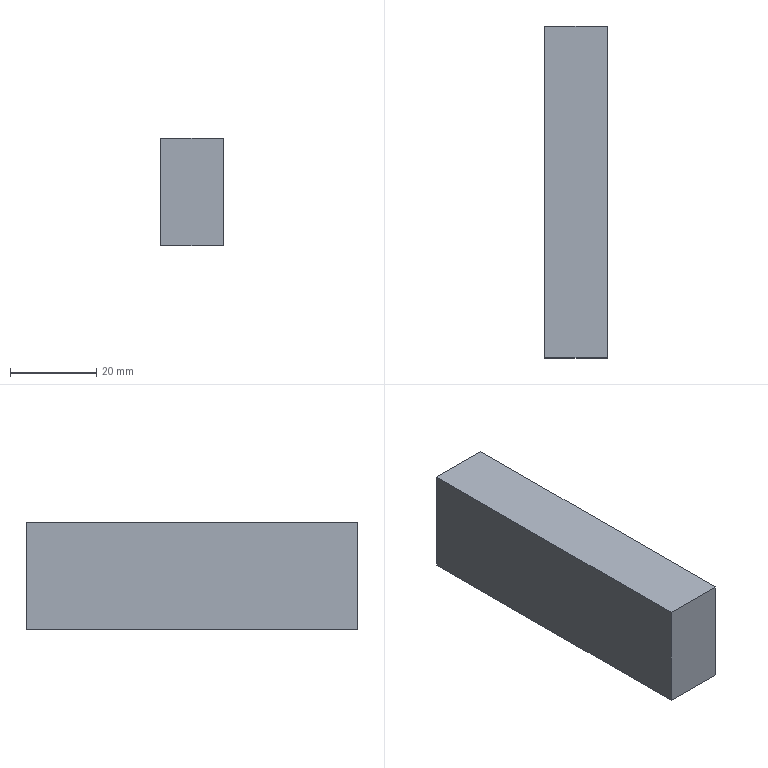Part | SolidWorks | features Extrusion 1 | 1 solid | 6 faces | box 14.5 x 77 x 25 mm | volume 27913 mm3 | plane 6
STEP:
#1=CARTESIAN_POINT('',(-7.25,38.5,0.));
#2=VERTEX_POINT('',#1);
#3=CARTESIAN_POINT('',(-7.25,-38.5,0.));
#4=VERTEX_POINT('',#3);
#5=CARTESIAN_POINT('',(-7.25,-38.5,0.));
#6=DIRECTION('',(0.,-1.,0.));
#7=VECTOR('',#6,1000.);
#8=LINE('',#5,#7);
#9=EDGE_CURVE('',#2,#4,#8,.T.);
#10=ORIENTED_EDGE('',*,*,#9,.T.);
#11=CARTESIAN_POINT('',(-7.25,-38.5,25.));
#12=VERTEX_POINT('',#11);
#13=CARTESIAN_POINT('',(-7.25,-38.5,25.));
#14=DIRECTION('',(0.,0.,-1.));
#15=VECTOR('',#14,1000.);
#16=LINE('',#13,#15);
#17=EDGE_CURVE('',#12,#4,#16,.T.);
#18=ORIENTED_EDGE('',*,*,#17,.F.);
#19=CARTESIAN_POINT('',(-7.25,38.5,25.));
#20=VERTEX_POINT('',#19);
#21=CARTESIAN_POINT('',(-7.25,-38.5,25.));
#22=DIRECTION('',(0.,-1.,0.));
#23=VECTOR('',#22,1000.);
#24=LINE('',#21,#23);
#25=EDGE_CURVE('',#20,#12,#24,.T.);
#26=ORIENTED_EDGE('',*,*,#25,.F.);
#27=CARTESIAN_POINT('',(-7.25,38.5,25.));
#28=DIRECTION('',(0.,0.,-1.));
#29=VECTOR('',#28,1000.);
#30=LINE('',#27,#29);
#31=EDGE_CURVE('',#20,#2,#30,.T.);
#32=ORIENTED_EDGE('',*,*,#31,.T.);
#33=EDGE_LOOP('',(#10,#18,#26,#32));
#34=FACE_OUTER_BOUND('',#33,.T.);
#35=CARTESIAN_POINT('',(-7.25,-38.5,25.));
#36=DIRECTION('',(1.,0.,0.));
#37=DIRECTION('',(0.,1.,0.));
#38=AXIS2_PLACEMENT_3D('',#35,#36,#37);
#39=PLANE('',#38);
#40=ADVANCED_FACE('',(#34),#39,.F.);
#41=CARTESIAN_POINT('',(7.25,-38.5,0.));
#42=VERTEX_POINT('',#41);
#43=CARTESIAN_POINT('',(7.25,-38.5,0.));
#44=DIRECTION('',(1.,0.,0.));
#45=VECTOR('',#44,1000.);
#46=LINE('',#43,#45);
#47=EDGE_CURVE('',#4,#42,#46,.T.);
#48=ORIENTED_EDGE('',*,*,#47,.T.);
#49=CARTESIAN_POINT('',(7.25,-38.5,25.));
#50=VERTEX_POINT('',#49);
#51=CARTESIAN_POINT('',(7.25,-38.5,25.));
#52=DIRECTION('',(0.,0.,-1.));
#53=VECTOR('',#52,1000.);
#54=LINE('',#51,#53);
#55=EDGE_CURVE('',#50,#42,#54,.T.);
#56=ORIENTED_EDGE('',*,*,#55,.F.);
#57=CARTESIAN_POINT('',(7.25,-38.5,25.));
#58=DIRECTION('',(1.,0.,0.));
#59=VECTOR('',#58,1000.);
#60=LINE('',#57,#59);
#61=EDGE_CURVE('',#12,#50,#60,.T.);
#62=ORIENTED_EDGE('',*,*,#61,.F.);
#63=ORIENTED_EDGE('',*,*,#17,.T.);
#64=EDGE_LOOP('',(#48,#56,#62,#63));
#65=FACE_OUTER_BOUND('',#64,.T.);
#66=CARTESIAN_POINT('',(7.25,-38.5,25.));
#67=DIRECTION('',(0.,1.,0.));
#68=DIRECTION('',(0.,0.,1.));
#69=AXIS2_PLACEMENT_3D('',#66,#67,#68);
#70=PLANE('',#69);
#71=ADVANCED_FACE('',(#65),#70,.F.);
#72=CARTESIAN_POINT('',(7.25,38.5,0.));
#73=VERTEX_POINT('',#72);
#74=CARTESIAN_POINT('',(7.25,-38.5,0.));
#75=DIRECTION('',(0.,1.,0.));
#76=VECTOR('',#75,1000.);
#77=LINE('',#74,#76);
#78=EDGE_CURVE('',#42,#73,#77,.T.);
#79=ORIENTED_EDGE('',*,*,#78,.T.);
#80=CARTESIAN_POINT('',(7.25,38.5,25.));
#81=VERTEX_POINT('',#80);
#82=CARTESIAN_POINT('',(7.25,38.5,25.));
#83=DIRECTION('',(0.,0.,-1.));
#84=VECTOR('',#83,1000.);
#85=LINE('',#82,#84);
#86=EDGE_CURVE('',#81,#73,#85,.T.);
#87=ORIENTED_EDGE('',*,*,#86,.F.);
#88=CARTESIAN_POINT('',(7.25,-38.5,25.));
#89=DIRECTION('',(0.,1.,0.));
#90=VECTOR('',#89,1000.);
#91=LINE('',#88,#90);
#92=EDGE_CURVE('',#50,#81,#91,.T.);
#93=ORIENTED_EDGE('',*,*,#92,.F.);
#94=ORIENTED_EDGE('',*,*,#55,.T.);
#95=EDGE_LOOP('',(#79,#87,#93,#94));
#96=FACE_OUTER_BOUND('',#95,.T.);
#97=CARTESIAN_POINT('',(7.25,-38.5,25.));
#98=DIRECTION('',(-1.,0.,0.));
#99=DIRECTION('',(0.,0.,1.));
#100=AXIS2_PLACEMENT_3D('',#97,#98,#99);
#101=PLANE('',#100);
#102=ADVANCED_FACE('',(#96),#101,.F.);
#103=CARTESIAN_POINT('',(7.25,38.5,0.));
#104=DIRECTION('',(-1.,0.,0.));
#105=VECTOR('',#104,1000.);
#106=LINE('',#103,#105);
#107=EDGE_CURVE('',#73,#2,#106,.T.);
#108=ORIENTED_EDGE('',*,*,#107,.T.);
#109=ORIENTED_EDGE('',*,*,#31,.F.);
#110=CARTESIAN_POINT('',(7.25,38.5,25.));
#111=DIRECTION('',(-1.,0.,0.));
#112=VECTOR('',#111,1000.);
#113=LINE('',#110,#112);
#114=EDGE_CURVE('',#81,#20,#113,.T.);
#115=ORIENTED_EDGE('',*,*,#114,.F.);
#116=ORIENTED_EDGE('',*,*,#86,.T.);
#117=EDGE_LOOP('',(#108,#109,#115,#116));
#118=FACE_OUTER_BOUND('',#117,.T.);
#119=CARTESIAN_POINT('',(7.25,38.5,25.));
#120=DIRECTION('',(0.,-1.,0.));
#121=DIRECTION('',(0.,0.,-1.));
#122=AXIS2_PLACEMENT_3D('',#119,#120,#121);
#123=PLANE('',#122);
#124=ADVANCED_FACE('',(#118),#123,.F.);
#125=ORIENTED_EDGE('',*,*,#25,.T.);
#126=ORIENTED_EDGE('',*,*,#61,.T.);
#127=ORIENTED_EDGE('',*,*,#92,.T.);
#128=ORIENTED_EDGE('',*,*,#114,.T.);
#129=EDGE_LOOP('',(#125,#126,#127,#128));
#130=FACE_OUTER_BOUND('',#129,.T.);
#131=CARTESIAN_POINT('',(0.,0.,25.));
#132=DIRECTION('',(0.,0.,1.));
#133=DIRECTION('',(1.,0.,0.));
#134=AXIS2_PLACEMENT_3D('',#131,#132,#133);
#135=PLANE('',#134);
#136=ADVANCED_FACE('',(#130),#135,.T.);
#137=ORIENTED_EDGE('',*,*,#9,.F.);
#138=ORIENTED_EDGE('',*,*,#107,.F.);
#139=ORIENTED_EDGE('',*,*,#78,.F.);
#140=ORIENTED_EDGE('',*,*,#47,.F.);
#141=EDGE_LOOP('',(#137,#138,#139,#140));
#142=FACE_OUTER_BOUND('',#141,.T.);
#143=CARTESIAN_POINT('',(0.,0.,0.));
#144=DIRECTION('',(0.,0.,1.));
#145=DIRECTION('',(1.,0.,0.));
#146=AXIS2_PLACEMENT_3D('',#143,#144,#145);
#147=PLANE('',#146);
#148=ADVANCED_FACE('',(#142),#147,.F.);
#149=CLOSED_SHELL('',(#40,#71,#102,#124,#136,#148));
#150=MANIFOLD_SOLID_BREP('',#149);
#151=CARTESIAN_POINT('',(0.,0.,0.));
#152=DIRECTION('',(0.,0.,1.));
#153=DIRECTION('',(1.,0.,0.));
#154=AXIS2_PLACEMENT_3D('',#151,#152,#153);
#155=(LENGTH_UNIT()NAMED_UNIT(*)SI_UNIT(.MILLI.,.METRE.));
#156=UNCERTAINTY_MEASURE_WITH_UNIT(LENGTH_MEASURE(0.00001),#155,'','');
#157=(NAMED_UNIT(*)PLANE_ANGLE_UNIT()SI_UNIT($,.RADIAN.));
#158=(NAMED_UNIT(*)SI_UNIT($,.STERADIAN.)SOLID_ANGLE_UNIT());
#159=(GEOMETRIC_REPRESENTATION_CONTEXT(3)GLOBAL_UNCERTAINTY_ASSIGNED_CONTEXT((#156))GLOBAL_UNIT_ASSIGNED_CONTEXT((#155,#157,#158))REPRESENTATION_CONTEXT('',''));
#160=ADVANCED_BREP_SHAPE_REPRESENTATION('',(#150,#154),#159);